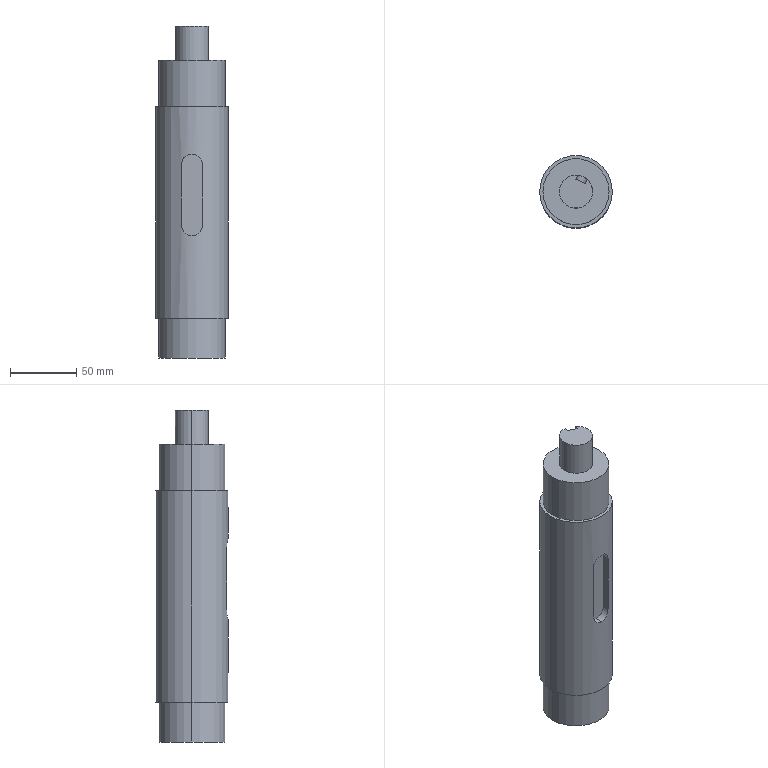Part | SolidWorks | features Cut 1, ICE 1, Revolution 1 | 1 solid | 23 faces | box 55 x 55 x 251.5 mm | volume 515825 mm3 | cylinder 12 | plane 11 | commonest cylinder face diameters 50 x4 16 x3 25 x2 55 x2 8 x1
STEP:
#1=CARTESIAN_POINT('',(0.,-21.5,58.5));
#2=VERTEX_POINT('',#1);
#3=CARTESIAN_POINT('',(8.,-21.5,66.5));
#4=VERTEX_POINT('',#3);
#5=CARTESIAN_POINT('',(0.,-21.5,66.5));
#6=DIRECTION('',(0.,-1.,0.));
#7=DIRECTION('',(0.,0.,-1.));
#8=AXIS2_PLACEMENT_3D('',#5,#6,#7);
#9=CIRCLE('',#8,8.);
#10=EDGE_CURVE('',#2,#4,#9,.T.);
#11=ORIENTED_EDGE('',*,*,#10,.F.);
#12=CARTESIAN_POINT('',(0.,-27.5,58.5));
#13=VERTEX_POINT('',#12);
#14=CARTESIAN_POINT('',(0.,-21.5,58.5));
#15=DIRECTION('',(0.,-1.,0.));
#16=VECTOR('',#15,1000.);
#17=LINE('',#14,#16);
#18=EDGE_CURVE('',#2,#13,#17,.T.);
#19=ORIENTED_EDGE('',*,*,#18,.T.);
#20=CARTESIAN_POINT('',(8.,-26.311,66.5));
#21=VERTEX_POINT('',#20);
#22=CARTESIAN_POINT('',(0.,-27.5,58.5));
#23=CARTESIAN_POINT('',(0.5246,-27.5,58.5));
#24=CARTESIAN_POINT('',(1.057,-27.484,58.553));
#25=CARTESIAN_POINT('',(2.085,-27.426,58.759));
#26=CARTESIAN_POINT('',(2.585,-27.383,58.911));
#27=CARTESIAN_POINT('',(3.313,-27.301,59.214));
#28=CARTESIAN_POINT('',(3.552,-27.271,59.327));
#29=CARTESIAN_POINT('',(4.012,-27.207,59.574));
#30=CARTESIAN_POINT('',(4.235,-27.173,59.708));
#31=CARTESIAN_POINT('',(4.666,-27.102,59.997));
#32=CARTESIAN_POINT('',(4.875,-27.065,60.152));
#33=CARTESIAN_POINT('',(5.278,-26.99,60.482));
#34=CARTESIAN_POINT('',(5.473,-26.951,60.659));
#35=CARTESIAN_POINT('',(6.027,-26.834,61.213));
#36=CARTESIAN_POINT('',(6.356,-26.757,61.614));
#37=CARTESIAN_POINT('',(6.934,-26.613,62.477));
#38=CARTESIAN_POINT('',(7.186,-26.545,62.945));
#39=CARTESIAN_POINT('',(7.586,-26.434,63.908));
#40=CARTESIAN_POINT('',(7.739,-26.389,64.406));
#41=CARTESIAN_POINT('',(7.895,-26.342,65.18));
#42=CARTESIAN_POINT('',(7.934,-26.331,65.443));
#43=CARTESIAN_POINT('',(7.987,-26.315,65.97));
#44=CARTESIAN_POINT('',(8.,-26.311,66.234));
#45=CARTESIAN_POINT('',(8.,-26.311,66.5));
#46=B_SPLINE_CURVE_WITH_KNOTS('',3,(#22,#23,#24,#25,#26,#27,#28,#29,#30,#31,#32,#33,#34,#35,#36,#37,#38,#39,#40,#41,#42,#43,#44,#45),.UNSPECIFIED.,.F.,.F.,(4,2,2,2,2,2,2,2,2,2,2,4),(0.01258,0.01415,0.01572,0.0165,0.01729,0.01807,0.01886,0.02043,0.022,0.02357,0.02435,0.02514),.UNSPECIFIED.);
#47=EDGE_CURVE('',#13,#21,#46,.T.);
#48=ORIENTED_EDGE('',*,*,#47,.T.);
#49=CARTESIAN_POINT('',(8.,-21.5,66.5));
#50=DIRECTION('',(0.,-1.,0.));
#51=VECTOR('',#50,1000.);
#52=LINE('',#49,#51);
#53=EDGE_CURVE('',#4,#21,#52,.T.);
#54=ORIENTED_EDGE('',*,*,#53,.F.);
#55=EDGE_LOOP('',(#11,#19,#48,#54));
#56=FACE_OUTER_BOUND('',#55,.T.);
#57=CARTESIAN_POINT('',(0.,-21.5,66.5));
#58=DIRECTION('',(0.,-1.,0.));
#59=DIRECTION('',(0.,0.,-1.));
#60=AXIS2_PLACEMENT_3D('',#57,#58,#59);
#61=CYLINDRICAL_SURFACE('',#60,8.);
#62=ADVANCED_FACE('',(#56),#61,.F.);
#63=CARTESIAN_POINT('',(-25.,0.,191.5));
#64=VERTEX_POINT('',#63);
#65=CARTESIAN_POINT('',(25.,0.,191.5));
#66=VERTEX_POINT('',#65);
#67=CARTESIAN_POINT('',(0.,0.,191.5));
#68=DIRECTION('',(0.,0.,-1.));
#69=DIRECTION('',(-1.,0.,0.));
#70=AXIS2_PLACEMENT_3D('',#67,#68,#69);
#71=CIRCLE('',#70,25.);
#72=EDGE_CURVE('',#64,#66,#71,.T.);
#73=ORIENTED_EDGE('',*,*,#72,.T.);
#74=CARTESIAN_POINT('',(25.,0.,156.5));
#75=VERTEX_POINT('',#74);
#76=CARTESIAN_POINT('',(25.,0.,0.));
#77=DIRECTION('',(0.,0.,-1.));
#78=VECTOR('',#77,1000.);
#79=LINE('',#76,#78);
#80=EDGE_CURVE('',#66,#75,#79,.T.);
#81=ORIENTED_EDGE('',*,*,#80,.T.);
#82=CARTESIAN_POINT('',(-25.,0.,156.5));
#83=VERTEX_POINT('',#82);
#84=CARTESIAN_POINT('',(0.,0.,156.5));
#85=DIRECTION('',(0.,0.,-1.));
#86=DIRECTION('',(-1.,0.,0.));
#87=AXIS2_PLACEMENT_3D('',#84,#85,#86);
#88=CIRCLE('',#87,25.);
#89=EDGE_CURVE('',#83,#75,#88,.T.);
#90=ORIENTED_EDGE('',*,*,#89,.F.);
#91=CARTESIAN_POINT('',(-25.,0.,0.));
#92=DIRECTION('',(0.,0.,-1.));
#93=VECTOR('',#92,1000.);
#94=LINE('',#91,#93);
#95=EDGE_CURVE('',#64,#83,#94,.T.);
#96=ORIENTED_EDGE('',*,*,#95,.F.);
#97=EDGE_LOOP('',(#73,#81,#90,#96));
#98=FACE_OUTER_BOUND('',#97,.T.);
#99=CARTESIAN_POINT('',(0.,0.,0.));
#100=DIRECTION('',(0.,0.,-1.));
#101=DIRECTION('',(-1.,0.,0.));
#102=AXIS2_PLACEMENT_3D('',#99,#100,#101);
#103=CYLINDRICAL_SURFACE('',#102,25.);
#104=ADVANCED_FACE('',(#98),#103,.T.);
#105=CARTESIAN_POINT('',(-27.5,0.,156.5));
#106=VERTEX_POINT('',#105);
#107=CARTESIAN_POINT('',(27.5,0.,156.5));
#108=VERTEX_POINT('',#107);
#109=CARTESIAN_POINT('',(0.,0.,156.5));
#110=DIRECTION('',(0.,0.,-1.));
#111=DIRECTION('',(-1.,0.,0.));
#112=AXIS2_PLACEMENT_3D('',#109,#110,#111);
#113=CIRCLE('',#112,27.5);
#114=EDGE_CURVE('',#106,#108,#113,.T.);
#115=ORIENTED_EDGE('',*,*,#114,.T.);
#116=CARTESIAN_POINT('',(27.5,0.,-4.));
#117=VERTEX_POINT('',#116);
#118=CARTESIAN_POINT('',(27.5,0.,0.));
#119=DIRECTION('',(0.,0.,-1.));
#120=VECTOR('',#119,1000.);
#121=LINE('',#118,#120);
#122=EDGE_CURVE('',#108,#117,#121,.T.);
#123=ORIENTED_EDGE('',*,*,#122,.T.);
#124=CARTESIAN_POINT('',(-27.5,0.,-4.));
#125=VERTEX_POINT('',#124);
#126=CARTESIAN_POINT('',(0.,0.,-4.));
#127=DIRECTION('',(0.,0.,-1.));
#128=DIRECTION('',(-1.,0.,0.));
#129=AXIS2_PLACEMENT_3D('',#126,#127,#128);
#130=CIRCLE('',#129,27.5);
#131=EDGE_CURVE('',#125,#117,#130,.T.);
#132=ORIENTED_EDGE('',*,*,#131,.F.);
#133=CARTESIAN_POINT('',(-27.5,0.,0.));
#134=DIRECTION('',(0.,0.,-1.));
#135=VECTOR('',#134,1000.);
#136=LINE('',#133,#135);
#137=EDGE_CURVE('',#106,#125,#136,.T.);
#138=ORIENTED_EDGE('',*,*,#137,.F.);
#139=EDGE_LOOP('',(#115,#123,#132,#138));
#140=FACE_OUTER_BOUND('',#139,.T.);
#141=CARTESIAN_POINT('',(0.,0.,0.));
#142=DIRECTION('',(0.,0.,-1.));
#143=DIRECTION('',(-1.,0.,0.));
#144=AXIS2_PLACEMENT_3D('',#141,#142,#143);
#145=CYLINDRICAL_SURFACE('',#144,27.5);
#146=ADVANCED_FACE('',(#140),#145,.T.);
#147=CARTESIAN_POINT('',(-25.,0.,-4.));
#148=VERTEX_POINT('',#147);
#149=CARTESIAN_POINT('',(25.,0.,-4.));
#150=VERTEX_POINT('',#149);
#151=CARTESIAN_POINT('',(0.,0.,-4.));
#152=DIRECTION('',(0.,0.,-1.));
#153=DIRECTION('',(-1.,0.,0.));
#154=AXIS2_PLACEMENT_3D('',#151,#152,#153);
#155=CIRCLE('',#154,25.);
#156=EDGE_CURVE('',#148,#150,#155,.T.);
#157=ORIENTED_EDGE('',*,*,#156,.T.);
#158=CARTESIAN_POINT('',(25.,0.,-34.));
#159=VERTEX_POINT('',#158);
#160=CARTESIAN_POINT('',(25.,0.,0.));
#161=DIRECTION('',(0.,0.,-1.));
#162=VECTOR('',#161,1000.);
#163=LINE('',#160,#162);
#164=EDGE_CURVE('',#150,#159,#163,.T.);
#165=ORIENTED_EDGE('',*,*,#164,.T.);
#166=CARTESIAN_POINT('',(-25.,0.,-34.));
#167=VERTEX_POINT('',#166);
#168=CARTESIAN_POINT('',(0.,0.,-34.));
#169=DIRECTION('',(0.,0.,-1.));
#170=DIRECTION('',(-1.,0.,0.));
#171=AXIS2_PLACEMENT_3D('',#168,#169,#170);
#172=CIRCLE('',#171,25.);
#173=EDGE_CURVE('',#167,#159,#172,.T.);
#174=ORIENTED_EDGE('',*,*,#173,.F.);
#175=CARTESIAN_POINT('',(-25.,0.,0.));
#176=DIRECTION('',(0.,0.,-1.));
#177=VECTOR('',#176,1000.);
#178=LINE('',#175,#177);
#179=EDGE_CURVE('',#148,#167,#178,.T.);
#180=ORIENTED_EDGE('',*,*,#179,.F.);
#181=EDGE_LOOP('',(#157,#165,#174,#180));
#182=FACE_OUTER_BOUND('',#181,.T.);
#183=CARTESIAN_POINT('',(0.,0.,0.));
#184=DIRECTION('',(0.,0.,-1.));
#185=DIRECTION('',(-1.,0.,0.));
#186=AXIS2_PLACEMENT_3D('',#183,#184,#185);
#187=CYLINDRICAL_SURFACE('',#186,25.);
#188=ADVANCED_FACE('',(#182),#187,.T.);
#189=CARTESIAN_POINT('',(8.598,9.073,217.5));
#190=VERTEX_POINT('',#189);
#191=CARTESIAN_POINT('',(12.5,0.,217.5));
#192=VERTEX_POINT('',#191);
#193=CARTESIAN_POINT('',(0.,0.,217.5));
#194=DIRECTION('',(0.,0.,-1.));
#195=DIRECTION('',(-1.,0.,0.));
#196=AXIS2_PLACEMENT_3D('',#193,#194,#195);
#197=CIRCLE('',#196,12.5);
#198=EDGE_CURVE('',#190,#192,#197,.T.);
#199=ORIENTED_EDGE('',*,*,#198,.T.);
#200=CARTESIAN_POINT('',(12.5,0.,191.5));
#201=VERTEX_POINT('',#200);
#202=CARTESIAN_POINT('',(12.5,0.,0.));
#203=DIRECTION('',(0.,0.,-1.));
#204=VECTOR('',#203,1000.);
#205=LINE('',#202,#204);
#206=EDGE_CURVE('',#192,#201,#205,.T.);
#207=ORIENTED_EDGE('',*,*,#206,.T.);
#208=CARTESIAN_POINT('',(-12.5,0.,191.5));
#209=VERTEX_POINT('',#208);
#210=CARTESIAN_POINT('',(0.,0.,191.5));
#211=DIRECTION('',(0.,0.,-1.));
#212=DIRECTION('',(-1.,0.,0.));
#213=AXIS2_PLACEMENT_3D('',#210,#211,#212);
#214=CIRCLE('',#213,12.5);
#215=EDGE_CURVE('',#209,#201,#214,.T.);
#216=ORIENTED_EDGE('',*,*,#215,.F.);
#217=CARTESIAN_POINT('',(-12.5,0.,217.5));
#218=VERTEX_POINT('',#217);
#219=CARTESIAN_POINT('',(-12.5,0.,0.));
#220=DIRECTION('',(0.,0.,-1.));
#221=VECTOR('',#220,1000.);
#222=LINE('',#219,#221);
#223=EDGE_CURVE('',#218,#209,#222,.T.);
#224=ORIENTED_EDGE('',*,*,#223,.F.);
#225=CARTESIAN_POINT('',(1.336,12.428,217.5));
#226=VERTEX_POINT('',#225);
#227=CARTESIAN_POINT('',(0.,0.,217.5));
#228=DIRECTION('',(0.,0.,-1.));
#229=DIRECTION('',(-1.,0.,0.));
#230=AXIS2_PLACEMENT_3D('',#227,#228,#229);
#231=CIRCLE('',#230,12.5);
#232=EDGE_CURVE('',#218,#226,#231,.T.);
#233=ORIENTED_EDGE('',*,*,#232,.T.);
#234=CARTESIAN_POINT('',(1.336,12.428,200.5));
#235=VERTEX_POINT('',#234);
#236=CARTESIAN_POINT('',(1.336,12.428,0.));
#237=DIRECTION('',(0.,0.,-1.));
#238=VECTOR('',#237,1000.);
#239=LINE('',#236,#238);
#240=EDGE_CURVE('',#226,#235,#239,.T.);
#241=ORIENTED_EDGE('',*,*,#240,.T.);
#242=CARTESIAN_POINT('',(8.598,9.073,200.5));
#243=VERTEX_POINT('',#242);
#244=CARTESIAN_POINT('',(1.336,12.428,200.5));
#245=CARTESIAN_POINT('',(1.336,12.428,200.234));
#246=CARTESIAN_POINT('',(1.364,12.426,199.973));
#247=CARTESIAN_POINT('',(1.471,12.413,199.459));
#248=CARTESIAN_POINT('',(1.552,12.404,199.204));
#249=CARTESIAN_POINT('',(1.761,12.376,198.721));
#250=CARTESIAN_POINT('',(1.888,12.358,198.492));
#251=CARTESIAN_POINT('',(2.185,12.309,198.059));
#252=CARTESIAN_POINT('',(2.355,12.278,197.855));
#253=CARTESIAN_POINT('',(2.723,12.201,197.489));
#254=CARTESIAN_POINT('',(2.923,12.156,197.324));
#255=CARTESIAN_POINT('',(3.352,12.044,197.031));
#256=CARTESIAN_POINT('',(3.576,11.98,196.908));
#257=CARTESIAN_POINT('',(4.037,11.833,196.708));
#258=CARTESIAN_POINT('',(4.277,11.748,196.63));
#259=CARTESIAN_POINT('',(4.76,11.561,196.526));
#260=CARTESIAN_POINT('',(5.001,11.459,196.5));
#261=CARTESIAN_POINT('',(5.478,11.239,196.5));
#262=CARTESIAN_POINT('',(5.717,11.119,196.526));
#263=CARTESIAN_POINT('',(6.17,10.874,196.629));
#264=CARTESIAN_POINT('',(6.387,10.748,196.705));
#265=CARTESIAN_POINT('',(6.804,10.489,196.907));
#266=CARTESIAN_POINT('',(6.999,10.359,197.031));
#267=CARTESIAN_POINT('',(7.358,10.108,197.32));
#268=CARTESIAN_POINT('',(7.525,9.983,197.487));
#269=CARTESIAN_POINT('',(7.823,9.751,197.855));
#270=CARTESIAN_POINT('',(7.955,9.643,198.055));
#271=CARTESIAN_POINT('',(8.184,9.449,198.487));
#272=CARTESIAN_POINT('',(8.283,9.363,198.72));
#273=CARTESIAN_POINT('',(8.439,9.222,199.202));
#274=CARTESIAN_POINT('',(8.498,9.167,199.451));
#275=CARTESIAN_POINT('',(8.578,9.092,199.968));
#276=CARTESIAN_POINT('',(8.598,9.073,200.234));
#277=CARTESIAN_POINT('',(8.598,9.073,200.5));
#278=B_SPLINE_CURVE_WITH_KNOTS('',3,(#244,#245,#246,#247,#248,#249,#250,#251,#252,#253,#254,#255,#256,#257,#258,#259,#260,#261,#262,#263,#264,#265,#266,#267,#268,#269,#270,#271,#272,#273,#274,#275,#276,#277),.UNSPECIFIED.,.F.,.F.,(4,2,2,2,2,2,2,2,2,2,2,2,2,2,2,2,4),(0.,0.0007865,0.001573,0.00236,0.003146,0.003933,0.004719,0.005506,0.006292,0.007079,0.007865,0.008652,0.009438,0.01022,0.01101,0.0118,0.01258),.UNSPECIFIED.);
#279=EDGE_CURVE('',#235,#243,#278,.T.);
#280=ORIENTED_EDGE('',*,*,#279,.T.);
#281=CARTESIAN_POINT('',(8.598,9.073,0.));
#282=DIRECTION('',(0.,0.,1.));
#283=VECTOR('',#282,1000.);
#284=LINE('',#281,#283);
#285=EDGE_CURVE('',#243,#190,#284,.T.);
#286=ORIENTED_EDGE('',*,*,#285,.T.);
#287=EDGE_LOOP('',(#199,#207,#216,#224,#233,#241,#280,#286));
#288=FACE_OUTER_BOUND('',#287,.T.);
#289=CARTESIAN_POINT('',(0.,0.,0.));
#290=DIRECTION('',(0.,0.,-1.));
#291=DIRECTION('',(-1.,0.,0.));
#292=AXIS2_PLACEMENT_3D('',#289,#290,#291);
#293=CYLINDRICAL_SURFACE('',#292,12.5);
#294=ADVANCED_FACE('',(#288),#293,.T.);
#295=ORIENTED_EDGE('',*,*,#206,.F.);
#296=CARTESIAN_POINT('',(0.,0.,217.5));
#297=DIRECTION('',(0.,0.,-1.));
#298=DIRECTION('',(-1.,0.,0.));
#299=AXIS2_PLACEMENT_3D('',#296,#297,#298);
#300=CIRCLE('',#299,12.5);
#301=EDGE_CURVE('',#192,#218,#300,.T.);
#302=ORIENTED_EDGE('',*,*,#301,.T.);
#303=ORIENTED_EDGE('',*,*,#223,.T.);
#304=CARTESIAN_POINT('',(0.,0.,191.5));
#305=DIRECTION('',(0.,0.,-1.));
#306=DIRECTION('',(-1.,0.,0.));
#307=AXIS2_PLACEMENT_3D('',#304,#305,#306);
#308=CIRCLE('',#307,12.5);
#309=EDGE_CURVE('',#201,#209,#308,.T.);
#310=ORIENTED_EDGE('',*,*,#309,.F.);
#311=EDGE_LOOP('',(#295,#302,#303,#310));
#312=FACE_OUTER_BOUND('',#311,.T.);
#313=CARTESIAN_POINT('',(0.,0.,0.));
#314=DIRECTION('',(0.,0.,-1.));
#315=DIRECTION('',(-1.,0.,0.));
#316=AXIS2_PLACEMENT_3D('',#313,#314,#315);
#317=CYLINDRICAL_SURFACE('',#316,12.5);
#318=ADVANCED_FACE('',(#312),#317,.T.);
#319=CARTESIAN_POINT('',(-0.06596,9.394,217.5));
#320=VERTEX_POINT('',#319);
#321=CARTESIAN_POINT('',(7.196,6.038,217.5));
#322=VERTEX_POINT('',#321);
#323=CARTESIAN_POINT('',(-6.736,12.476,217.5));
#324=DIRECTION('',(0.9078,-0.4194,0.));
#325=VECTOR('',#324,1000.);
#326=LINE('',#323,#325);
#327=EDGE_CURVE('',#320,#322,#326,.T.);
#328=ORIENTED_EDGE('',*,*,#327,.F.);
#329=CARTESIAN_POINT('',(-5.83,-3.082,217.5));
#330=DIRECTION('',(0.4194,0.9078,0.));
#331=VECTOR('',#330,1000.);
#332=LINE('',#329,#331);
#333=EDGE_CURVE('',#320,#226,#332,.T.);
#334=ORIENTED_EDGE('',*,*,#333,.T.);
#335=ORIENTED_EDGE('',*,*,#232,.F.);
#336=ORIENTED_EDGE('',*,*,#301,.F.);
#337=ORIENTED_EDGE('',*,*,#198,.F.);
#338=CARTESIAN_POINT('',(1.432,-6.437,217.5));
#339=DIRECTION('',(-0.4194,-0.9078,0.));
#340=VECTOR('',#339,1000.);
#341=LINE('',#338,#340);
#342=EDGE_CURVE('',#190,#322,#341,.T.);
#343=ORIENTED_EDGE('',*,*,#342,.T.);
#344=EDGE_LOOP('',(#328,#334,#335,#336,#337,#343));
#345=FACE_OUTER_BOUND('',#344,.T.);
#346=CARTESIAN_POINT('',(-12.5,0.,217.5));
#347=DIRECTION('',(0.,0.,1.));
#348=DIRECTION('',(1.,0.,0.));
#349=AXIS2_PLACEMENT_3D('',#346,#347,#348);
#350=PLANE('',#349);
#351=ADVANCED_FACE('',(#345),#350,.T.);
#352=ORIENTED_EDGE('',*,*,#173,.T.);
#353=CARTESIAN_POINT('',(0.,0.,-34.));
#354=DIRECTION('',(0.,0.,-1.));
#355=DIRECTION('',(-1.,0.,0.));
#356=AXIS2_PLACEMENT_3D('',#353,#354,#355);
#357=CIRCLE('',#356,25.);
#358=EDGE_CURVE('',#159,#167,#357,.T.);
#359=ORIENTED_EDGE('',*,*,#358,.T.);
#360=EDGE_LOOP('',(#352,#359));
#361=FACE_OUTER_BOUND('',#360,.T.);
#362=CARTESIAN_POINT('',(-25.,0.,-34.));
#363=DIRECTION('',(0.,0.,-1.));
#364=DIRECTION('',(-1.,0.,0.));
#365=AXIS2_PLACEMENT_3D('',#362,#363,#364);
#366=PLANE('',#365);
#367=ADVANCED_FACE('',(#361),#366,.T.);
#368=ORIENTED_EDGE('',*,*,#164,.F.);
#369=CARTESIAN_POINT('',(0.,0.,-4.));
#370=DIRECTION('',(0.,0.,-1.));
#371=DIRECTION('',(-1.,0.,0.));
#372=AXIS2_PLACEMENT_3D('',#369,#370,#371);
#373=CIRCLE('',#372,25.);
#374=EDGE_CURVE('',#150,#148,#373,.T.);
#375=ORIENTED_EDGE('',*,*,#374,.T.);
#376=ORIENTED_EDGE('',*,*,#179,.T.);
#377=ORIENTED_EDGE('',*,*,#358,.F.);
#378=EDGE_LOOP('',(#368,#375,#376,#377));
#379=FACE_OUTER_BOUND('',#378,.T.);
#380=CARTESIAN_POINT('',(0.,0.,0.));
#381=DIRECTION('',(0.,0.,-1.));
#382=DIRECTION('',(-1.,0.,0.));
#383=AXIS2_PLACEMENT_3D('',#380,#381,#382);
#384=CYLINDRICAL_SURFACE('',#383,25.);
#385=ADVANCED_FACE('',(#379),#384,.T.);
#386=ORIENTED_EDGE('',*,*,#131,.T.);
#387=CARTESIAN_POINT('',(0.,0.,-4.));
#388=DIRECTION('',(0.,0.,-1.));
#389=DIRECTION('',(-1.,0.,0.));
#390=AXIS2_PLACEMENT_3D('',#387,#388,#389);
#391=CIRCLE('',#390,27.5);
#392=EDGE_CURVE('',#117,#125,#391,.T.);
#393=ORIENTED_EDGE('',*,*,#392,.T.);
#394=EDGE_LOOP('',(#386,#393));
#395=FACE_OUTER_BOUND('',#394,.T.);
#396=ORIENTED_EDGE('',*,*,#156,.F.);
#397=ORIENTED_EDGE('',*,*,#374,.F.);
#398=EDGE_LOOP('',(#396,#397));
#399=FACE_BOUND('',#398,.T.);
#400=CARTESIAN_POINT('',(-25.,0.,-4.));
#401=DIRECTION('',(0.,0.,-1.));
#402=DIRECTION('',(-1.,0.,0.));
#403=AXIS2_PLACEMENT_3D('',#400,#401,#402);
#404=PLANE('',#403);
#405=ADVANCED_FACE('',(#395,#399),#404,.T.);
#406=ORIENTED_EDGE('',*,*,#122,.F.);
#407=CARTESIAN_POINT('',(0.,0.,156.5));
#408=DIRECTION('',(0.,0.,-1.));
#409=DIRECTION('',(-1.,0.,0.));
#410=AXIS2_PLACEMENT_3D('',#407,#408,#409);
#411=CIRCLE('',#410,27.5);
#412=EDGE_CURVE('',#108,#106,#411,.T.);
#413=ORIENTED_EDGE('',*,*,#412,.T.);
#414=ORIENTED_EDGE('',*,*,#137,.T.);
#415=ORIENTED_EDGE('',*,*,#392,.F.);
#416=EDGE_LOOP('',(#406,#413,#414,#415));
#417=FACE_OUTER_BOUND('',#416,.T.);
#418=CARTESIAN_POINT('',(8.,-26.311,112.5));
#419=VERTEX_POINT('',#418);
#420=CARTESIAN_POINT('',(-8.,-26.311,112.5));
#421=VERTEX_POINT('',#420);
#422=CARTESIAN_POINT('',(8.,-26.311,112.5));
#423=CARTESIAN_POINT('',(8.,-26.311,113.032));
#424=CARTESIAN_POINT('',(7.948,-26.327,113.554));
#425=CARTESIAN_POINT('',(7.794,-26.372,114.323));
#426=CARTESIAN_POINT('',(7.73,-26.391,114.577));
#427=CARTESIAN_POINT('',(7.577,-26.436,115.081));
#428=CARTESIAN_POINT('',(7.487,-26.461,115.331));
#429=CARTESIAN_POINT('',(7.185,-26.546,116.056));
#430=CARTESIAN_POINT('',(6.94,-26.612,116.514));
#431=CARTESIAN_POINT('',(6.504,-26.72,117.165));
#432=CARTESIAN_POINT('',(6.347,-26.758,117.376));
#433=CARTESIAN_POINT('',(6.015,-26.835,117.781));
#434=CARTESIAN_POINT('',(5.841,-26.873,117.973));
#435=CARTESIAN_POINT('',(5.29,-26.989,118.523));
#436=CARTESIAN_POINT('',(4.89,-27.065,118.853));
#437=CARTESIAN_POINT('',(4.016,-27.209,119.439));
#438=CARTESIAN_POINT('',(3.556,-27.273,119.685));
#439=CARTESIAN_POINT('',(2.835,-27.355,119.985));
#440=CARTESIAN_POINT('',(2.589,-27.379,120.074));
#441=CARTESIAN_POINT('',(2.087,-27.422,120.227));
#442=CARTESIAN_POINT('',(1.829,-27.44,120.293));
#443=CARTESIAN_POINT('',(1.054,-27.485,120.448));
#444=CARTESIAN_POINT('',(0.5326,-27.5,120.499));
#445=CARTESIAN_POINT('',(-0.5171,-27.5,120.501));
#446=CARTESIAN_POINT('',(-1.05,-27.485,120.448));
#447=CARTESIAN_POINT('',(-2.079,-27.426,120.243));
#448=CARTESIAN_POINT('',(-2.579,-27.383,120.091));
#449=CARTESIAN_POINT('',(-3.308,-27.301,119.789));
#450=CARTESIAN_POINT('',(-3.547,-27.271,119.675));
#451=CARTESIAN_POINT('',(-4.008,-27.207,119.429));
#452=CARTESIAN_POINT('',(-4.231,-27.173,119.295));
#453=CARTESIAN_POINT('',(-4.663,-27.103,119.006));
#454=CARTESIAN_POINT('',(-4.871,-27.066,118.851));
#455=CARTESIAN_POINT('',(-5.275,-26.99,118.52));
#456=CARTESIAN_POINT('',(-5.47,-26.951,118.343));
#457=CARTESIAN_POINT('',(-6.024,-26.835,117.789));
#458=CARTESIAN_POINT('',(-6.354,-26.758,117.389));
#459=CARTESIAN_POINT('',(-6.933,-26.613,116.525));
#460=CARTESIAN_POINT('',(-7.185,-26.546,116.057));
#461=CARTESIAN_POINT('',(-7.586,-26.434,115.094));
#462=CARTESIAN_POINT('',(-7.739,-26.389,114.595));
#463=CARTESIAN_POINT('',(-7.895,-26.343,113.821));
#464=CARTESIAN_POINT('',(-7.934,-26.331,113.558));
#465=CARTESIAN_POINT('',(-7.987,-26.315,113.03));
#466=CARTESIAN_POINT('',(-8.,-26.311,112.766));
#467=CARTESIAN_POINT('',(-8.,-26.311,112.5));
#468=B_SPLINE_CURVE_WITH_KNOTS('',3,(#422,#423,#424,#425,#426,#427,#428,#429,#430,#431,#432,#433,#434,#435,#436,#437,#438,#439,#440,#441,#442,#443,#444,#445,#446,#447,#448,#449,#450,#451,#452,#453,#454,#455,#456,#457,#458,#459,#460,#461,#462,#463,#464,#465,#466,#467),.UNSPECIFIED.,.F.,.F.,(4,2,2,2,2,2,2,2,2,2,2,2,2,2,2,2,2,2,2,2,2,2,4),(0.,0.001571,0.002357,0.003142,0.004714,0.005499,0.006285,0.007856,0.009427,0.01021,0.011,0.01257,0.01414,0.01571,0.0165,0.01728,0.01807,0.01885,0.02043,0.022,0.02357,0.02435,0.02514),.UNSPECIFIED.);
#469=EDGE_CURVE('',#419,#421,#468,.T.);
#470=ORIENTED_EDGE('',*,*,#469,.F.);
#471=CARTESIAN_POINT('',(8.,-26.311,0.));
#472=DIRECTION('',(0.,0.,1.));
#473=VECTOR('',#472,1000.);
#474=LINE('',#471,#473);
#475=EDGE_CURVE('',#21,#419,#474,.T.);
#476=ORIENTED_EDGE('',*,*,#475,.F.);
#477=ORIENTED_EDGE('',*,*,#47,.F.);
#478=CARTESIAN_POINT('',(-8.,-26.311,66.5));
#479=VERTEX_POINT('',#478);
#480=CARTESIAN_POINT('',(-8.,-26.311,66.5));
#481=CARTESIAN_POINT('',(-8.,-26.311,65.968));
#482=CARTESIAN_POINT('',(-7.947,-26.327,65.446));
#483=CARTESIAN_POINT('',(-7.794,-26.373,64.676));
#484=CARTESIAN_POINT('',(-7.73,-26.391,64.421));
#485=CARTESIAN_POINT('',(-7.576,-26.436,63.917));
#486=CARTESIAN_POINT('',(-7.486,-26.462,63.667));
#487=CARTESIAN_POINT('',(-7.184,-26.546,62.942));
#488=CARTESIAN_POINT('',(-6.938,-26.612,62.483));
#489=CARTESIAN_POINT('',(-6.503,-26.721,61.833));
#490=CARTESIAN_POINT('',(-6.345,-26.758,61.621));
#491=CARTESIAN_POINT('',(-6.013,-26.835,61.217));
#492=CARTESIAN_POINT('',(-5.838,-26.874,61.024));
#493=CARTESIAN_POINT('',(-5.287,-26.99,60.474));
#494=CARTESIAN_POINT('',(-4.886,-27.066,60.144));
#495=CARTESIAN_POINT('',(-4.012,-27.209,59.559));
#496=CARTESIAN_POINT('',(-3.551,-27.274,59.312));
#497=CARTESIAN_POINT('',(-2.829,-27.355,59.012));
#498=CARTESIAN_POINT('',(-2.583,-27.38,58.924));
#499=CARTESIAN_POINT('',(-2.081,-27.422,58.771));
#500=CARTESIAN_POINT('',(-1.822,-27.441,58.706));
#501=CARTESIAN_POINT('',(-1.047,-27.485,58.551));
#502=CARTESIAN_POINT('',(-0.5252,-27.5,58.5));
#503=CARTESIAN_POINT('',(0.,-27.5,58.5));
#504=B_SPLINE_CURVE_WITH_KNOTS('',3,(#480,#481,#482,#483,#484,#485,#486,#487,#488,#489,#490,#491,#492,#493,#494,#495,#496,#497,#498,#499,#500,#501,#502,#503),.UNSPECIFIED.,.F.,.F.,(4,2,2,2,2,2,2,2,2,2,2,4),(0.,0.001572,0.002358,0.003144,0.004717,0.005503,0.006289,0.007861,0.009433,0.01022,0.01101,0.01258),.UNSPECIFIED.);
#505=EDGE_CURVE('',#479,#13,#504,.T.);
#506=ORIENTED_EDGE('',*,*,#505,.F.);
#507=CARTESIAN_POINT('',(-8.,-26.311,0.));
#508=DIRECTION('',(0.,0.,-1.));
#509=VECTOR('',#508,1000.);
#510=LINE('',#507,#509);
#511=EDGE_CURVE('',#421,#479,#510,.T.);
#512=ORIENTED_EDGE('',*,*,#511,.F.);
#513=EDGE_LOOP('',(#470,#476,#477,#506,#512));
#514=FACE_BOUND('',#513,.T.);
#515=CARTESIAN_POINT('',(0.,0.,0.));
#516=DIRECTION('',(0.,0.,-1.));
#517=DIRECTION('',(-1.,0.,0.));
#518=AXIS2_PLACEMENT_3D('',#515,#516,#517);
#519=CYLINDRICAL_SURFACE('',#518,27.5);
#520=ADVANCED_FACE('',(#417,#514),#519,.T.);
#521=ORIENTED_EDGE('',*,*,#89,.T.);
#522=CARTESIAN_POINT('',(0.,0.,156.5));
#523=DIRECTION('',(0.,0.,-1.));
#524=DIRECTION('',(-1.,0.,0.));
#525=AXIS2_PLACEMENT_3D('',#522,#523,#524);
#526=CIRCLE('',#525,25.);
#527=EDGE_CURVE('',#75,#83,#526,.T.);
#528=ORIENTED_EDGE('',*,*,#527,.T.);
#529=EDGE_LOOP('',(#521,#528));
#530=FACE_BOUND('',#529,.T.);
#531=ORIENTED_EDGE('',*,*,#114,.F.);
#532=ORIENTED_EDGE('',*,*,#412,.F.);
#533=EDGE_LOOP('',(#531,#532));
#534=FACE_OUTER_BOUND('',#533,.T.);
#535=CARTESIAN_POINT('',(-27.5,0.,156.5));
#536=DIRECTION('',(0.,0.,1.));
#537=DIRECTION('',(1.,0.,0.));
#538=AXIS2_PLACEMENT_3D('',#535,#536,#537);
#539=PLANE('',#538);
#540=ADVANCED_FACE('',(#530,#534),#539,.T.);
#541=ORIENTED_EDGE('',*,*,#80,.F.);
#542=CARTESIAN_POINT('',(0.,0.,191.5));
#543=DIRECTION('',(0.,0.,-1.));
#544=DIRECTION('',(-1.,0.,0.));
#545=AXIS2_PLACEMENT_3D('',#542,#543,#544);
#546=CIRCLE('',#545,25.);
#547=EDGE_CURVE('',#66,#64,#546,.T.);
#548=ORIENTED_EDGE('',*,*,#547,.T.);
#549=ORIENTED_EDGE('',*,*,#95,.T.);
#550=ORIENTED_EDGE('',*,*,#527,.F.);
#551=EDGE_LOOP('',(#541,#548,#549,#550));
#552=FACE_OUTER_BOUND('',#551,.T.);
#553=CARTESIAN_POINT('',(0.,0.,0.));
#554=DIRECTION('',(0.,0.,-1.));
#555=DIRECTION('',(-1.,0.,0.));
#556=AXIS2_PLACEMENT_3D('',#553,#554,#555);
#557=CYLINDRICAL_SURFACE('',#556,25.);
#558=ADVANCED_FACE('',(#552),#557,.T.);
#559=ORIENTED_EDGE('',*,*,#215,.T.);
#560=ORIENTED_EDGE('',*,*,#309,.T.);
#561=EDGE_LOOP('',(#559,#560));
#562=FACE_BOUND('',#561,.T.);
#563=ORIENTED_EDGE('',*,*,#72,.F.);
#564=ORIENTED_EDGE('',*,*,#547,.F.);
#565=EDGE_LOOP('',(#563,#564));
#566=FACE_OUTER_BOUND('',#565,.T.);
#567=CARTESIAN_POINT('',(-25.,0.,191.5));
#568=DIRECTION('',(0.,0.,1.));
#569=DIRECTION('',(1.,0.,0.));
#570=AXIS2_PLACEMENT_3D('',#567,#568,#569);
#571=PLANE('',#570);
#572=ADVANCED_FACE('',(#562,#566),#571,.T.);
#573=ORIENTED_EDGE('',*,*,#18,.F.);
#574=CARTESIAN_POINT('',(-8.,-21.5,66.5));
#575=VERTEX_POINT('',#574);
#576=CARTESIAN_POINT('',(0.,-21.5,66.5));
#577=DIRECTION('',(0.,-1.,0.));
#578=DIRECTION('',(0.,0.,-1.));
#579=AXIS2_PLACEMENT_3D('',#576,#577,#578);
#580=CIRCLE('',#579,8.);
#581=EDGE_CURVE('',#575,#2,#580,.T.);
#582=ORIENTED_EDGE('',*,*,#581,.F.);
#583=CARTESIAN_POINT('',(-8.,-21.5,66.5));
#584=DIRECTION('',(0.,-1.,0.));
#585=VECTOR('',#584,1000.);
#586=LINE('',#583,#585);
#587=EDGE_CURVE('',#575,#479,#586,.T.);
#588=ORIENTED_EDGE('',*,*,#587,.T.);
#589=ORIENTED_EDGE('',*,*,#505,.T.);
#590=EDGE_LOOP('',(#573,#582,#588,#589));
#591=FACE_OUTER_BOUND('',#590,.T.);
#592=CARTESIAN_POINT('',(0.,-21.5,66.5));
#593=DIRECTION('',(0.,-1.,0.));
#594=DIRECTION('',(0.,0.,-1.));
#595=AXIS2_PLACEMENT_3D('',#592,#593,#594);
#596=CYLINDRICAL_SURFACE('',#595,8.);
#597=ADVANCED_FACE('',(#591),#596,.F.);
#598=ORIENTED_EDGE('',*,*,#511,.T.);
#599=ORIENTED_EDGE('',*,*,#587,.F.);
#600=CARTESIAN_POINT('',(-8.,-21.5,112.5));
#601=VERTEX_POINT('',#600);
#602=CARTESIAN_POINT('',(-8.,-21.5,66.5));
#603=DIRECTION('',(0.,0.,-1.));
#604=VECTOR('',#603,1000.);
#605=LINE('',#602,#604);
#606=EDGE_CURVE('',#601,#575,#605,.T.);
#607=ORIENTED_EDGE('',*,*,#606,.F.);
#608=CARTESIAN_POINT('',(-8.,-21.5,112.5));
#609=DIRECTION('',(0.,-1.,0.));
#610=VECTOR('',#609,1000.);
#611=LINE('',#608,#610);
#612=EDGE_CURVE('',#601,#421,#611,.T.);
#613=ORIENTED_EDGE('',*,*,#612,.T.);
#614=EDGE_LOOP('',(#598,#599,#607,#613));
#615=FACE_OUTER_BOUND('',#614,.T.);
#616=CARTESIAN_POINT('',(-8.,-21.5,66.5));
#617=DIRECTION('',(-1.,0.,0.));
#618=DIRECTION('',(0.,0.,1.));
#619=AXIS2_PLACEMENT_3D('',#616,#617,#618);
#620=PLANE('',#619);
#621=ADVANCED_FACE('',(#615),#620,.F.);
#622=CARTESIAN_POINT('',(8.,-21.5,112.5));
#623=VERTEX_POINT('',#622);
#624=CARTESIAN_POINT('',(8.,-21.5,112.5));
#625=DIRECTION('',(0.,-1.,0.));
#626=VECTOR('',#625,1000.);
#627=LINE('',#624,#626);
#628=EDGE_CURVE('',#623,#419,#627,.T.);
#629=ORIENTED_EDGE('',*,*,#628,.T.);
#630=ORIENTED_EDGE('',*,*,#469,.T.);
#631=ORIENTED_EDGE('',*,*,#612,.F.);
#632=CARTESIAN_POINT('',(0.,-21.5,112.5));
#633=DIRECTION('',(0.,-1.,0.));
#634=DIRECTION('',(0.,0.,-1.));
#635=AXIS2_PLACEMENT_3D('',#632,#633,#634);
#636=CIRCLE('',#635,8.);
#637=EDGE_CURVE('',#623,#601,#636,.T.);
#638=ORIENTED_EDGE('',*,*,#637,.F.);
#639=EDGE_LOOP('',(#629,#630,#631,#638));
#640=FACE_OUTER_BOUND('',#639,.T.);
#641=CARTESIAN_POINT('',(0.,-21.5,112.5));
#642=DIRECTION('',(0.,-1.,0.));
#643=DIRECTION('',(0.,0.,-1.));
#644=AXIS2_PLACEMENT_3D('',#641,#642,#643);
#645=CYLINDRICAL_SURFACE('',#644,8.);
#646=ADVANCED_FACE('',(#640),#645,.F.);
#647=ORIENTED_EDGE('',*,*,#475,.T.);
#648=ORIENTED_EDGE('',*,*,#628,.F.);
#649=CARTESIAN_POINT('',(8.,-21.5,66.5));
#650=DIRECTION('',(0.,0.,1.));
#651=VECTOR('',#650,1000.);
#652=LINE('',#649,#651);
#653=EDGE_CURVE('',#4,#623,#652,.T.);
#654=ORIENTED_EDGE('',*,*,#653,.F.);
#655=ORIENTED_EDGE('',*,*,#53,.T.);
#656=EDGE_LOOP('',(#647,#648,#654,#655));
#657=FACE_OUTER_BOUND('',#656,.T.);
#658=CARTESIAN_POINT('',(8.,-21.5,66.5));
#659=DIRECTION('',(1.,0.,0.));
#660=DIRECTION('',(0.,0.,-1.));
#661=AXIS2_PLACEMENT_3D('',#658,#659,#660);
#662=PLANE('',#661);
#663=ADVANCED_FACE('',(#657),#662,.F.);
#664=ORIENTED_EDGE('',*,*,#581,.T.);
#665=ORIENTED_EDGE('',*,*,#10,.T.);
#666=ORIENTED_EDGE('',*,*,#653,.T.);
#667=ORIENTED_EDGE('',*,*,#637,.T.);
#668=ORIENTED_EDGE('',*,*,#606,.T.);
#669=EDGE_LOOP('',(#664,#665,#666,#667,#668));
#670=FACE_OUTER_BOUND('',#669,.T.);
#671=CARTESIAN_POINT('',(0.,-21.5,66.5));
#672=DIRECTION('',(0.,-1.,0.));
#673=DIRECTION('',(0.,0.,-1.));
#674=AXIS2_PLACEMENT_3D('',#671,#672,#673);
#675=PLANE('',#674);
#676=ADVANCED_FACE('',(#670),#675,.T.);
#677=ORIENTED_EDGE('',*,*,#333,.F.);
#678=CARTESIAN_POINT('',(-0.06596,9.394,200.5));
#679=VERTEX_POINT('',#678);
#680=CARTESIAN_POINT('',(-0.06596,9.394,219.353));
#681=DIRECTION('',(0.,0.,-1.));
#682=VECTOR('',#681,1000.);
#683=LINE('',#680,#682);
#684=EDGE_CURVE('',#320,#679,#683,.T.);
#685=ORIENTED_EDGE('',*,*,#684,.T.);
#686=CARTESIAN_POINT('',(-0.06596,9.394,200.5));
#687=DIRECTION('',(0.4194,0.9078,0.));
#688=VECTOR('',#687,1000.);
#689=LINE('',#686,#688);
#690=EDGE_CURVE('',#679,#235,#689,.T.);
#691=ORIENTED_EDGE('',*,*,#690,.T.);
#692=ORIENTED_EDGE('',*,*,#240,.F.);
#693=EDGE_LOOP('',(#677,#685,#691,#692));
#694=FACE_OUTER_BOUND('',#693,.T.);
#695=CARTESIAN_POINT('',(-0.06596,9.394,219.353));
#696=DIRECTION('',(0.9078,-0.4194,0.));
#697=DIRECTION('',(0.4194,0.9078,0.));
#698=AXIS2_PLACEMENT_3D('',#695,#696,#697);
#699=PLANE('',#698);
#700=ADVANCED_FACE('',(#694),#699,.T.);
#701=ORIENTED_EDGE('',*,*,#690,.F.);
#702=CARTESIAN_POINT('',(7.196,6.038,200.5));
#703=VERTEX_POINT('',#702);
#704=CARTESIAN_POINT('',(3.565,7.716,200.5));
#705=DIRECTION('',(-0.4194,-0.9078,0.));
#706=DIRECTION('',(0.9078,-0.4194,0.));
#707=AXIS2_PLACEMENT_3D('',#704,#705,#706);
#708=CIRCLE('',#707,4.);
#709=EDGE_CURVE('',#679,#703,#708,.T.);
#710=ORIENTED_EDGE('',*,*,#709,.T.);
#711=CARTESIAN_POINT('',(7.196,6.038,200.5));
#712=DIRECTION('',(0.4194,0.9078,0.));
#713=VECTOR('',#712,1000.);
#714=LINE('',#711,#713);
#715=EDGE_CURVE('',#703,#243,#714,.T.);
#716=ORIENTED_EDGE('',*,*,#715,.T.);
#717=ORIENTED_EDGE('',*,*,#279,.F.);
#718=EDGE_LOOP('',(#701,#710,#716,#717));
#719=FACE_OUTER_BOUND('',#718,.T.);
#720=CARTESIAN_POINT('',(3.565,7.716,200.5));
#721=DIRECTION('',(0.4194,0.9078,0.));
#722=DIRECTION('',(-0.9078,0.4194,0.));
#723=AXIS2_PLACEMENT_3D('',#720,#721,#722);
#724=CYLINDRICAL_SURFACE('',#723,4.);
#725=ADVANCED_FACE('',(#719),#724,.F.);
#726=ORIENTED_EDGE('',*,*,#715,.F.);
#727=CARTESIAN_POINT('',(7.196,6.038,219.353));
#728=DIRECTION('',(0.,0.,1.));
#729=VECTOR('',#728,1000.);
#730=LINE('',#727,#729);
#731=EDGE_CURVE('',#703,#322,#730,.T.);
#732=ORIENTED_EDGE('',*,*,#731,.T.);
#733=ORIENTED_EDGE('',*,*,#342,.F.);
#734=ORIENTED_EDGE('',*,*,#285,.F.);
#735=EDGE_LOOP('',(#726,#732,#733,#734));
#736=FACE_OUTER_BOUND('',#735,.T.);
#737=CARTESIAN_POINT('',(7.196,6.038,219.353));
#738=DIRECTION('',(-0.9078,0.4194,0.));
#739=DIRECTION('',(-0.4194,-0.9078,0.));
#740=AXIS2_PLACEMENT_3D('',#737,#738,#739);
#741=PLANE('',#740);
#742=ADVANCED_FACE('',(#736),#741,.T.);
#743=ORIENTED_EDGE('',*,*,#327,.T.);
#744=ORIENTED_EDGE('',*,*,#731,.F.);
#745=ORIENTED_EDGE('',*,*,#709,.F.);
#746=ORIENTED_EDGE('',*,*,#684,.F.);
#747=EDGE_LOOP('',(#743,#744,#745,#746));
#748=FACE_OUTER_BOUND('',#747,.T.);
#749=CARTESIAN_POINT('',(3.565,7.716,219.353));
#750=DIRECTION('',(-0.4194,-0.9078,0.));
#751=DIRECTION('',(0.9078,-0.4194,0.));
#752=AXIS2_PLACEMENT_3D('',#749,#750,#751);
#753=PLANE('',#752);
#754=ADVANCED_FACE('',(#748),#753,.F.);
#755=CLOSED_SHELL('',(#62,#104,#146,#188,#294,#318,#351,#367,#385,#405,#520,#540,#558,#572,#597,#621,#646,#663,#676,#700,#725,#742,#754));
#756=MANIFOLD_SOLID_BREP('',#755);
#757=CARTESIAN_POINT('',(0.,0.,0.));
#758=DIRECTION('',(0.,0.,1.));
#759=DIRECTION('',(1.,0.,0.));
#760=AXIS2_PLACEMENT_3D('',#757,#758,#759);
#761=(LENGTH_UNIT()NAMED_UNIT(*)SI_UNIT(.MILLI.,.METRE.));
#762=UNCERTAINTY_MEASURE_WITH_UNIT(LENGTH_MEASURE(0.00001),#761,'','');
#763=(NAMED_UNIT(*)PLANE_ANGLE_UNIT()SI_UNIT($,.RADIAN.));
#764=(NAMED_UNIT(*)SI_UNIT($,.STERADIAN.)SOLID_ANGLE_UNIT());
#765=(GEOMETRIC_REPRESENTATION_CONTEXT(3)GLOBAL_UNCERTAINTY_ASSIGNED_CONTEXT((#762))GLOBAL_UNIT_ASSIGNED_CONTEXT((#761,#763,#764))REPRESENTATION_CONTEXT('',''));
#766=ADVANCED_BREP_SHAPE_REPRESENTATION('',(#756,#760),#765);